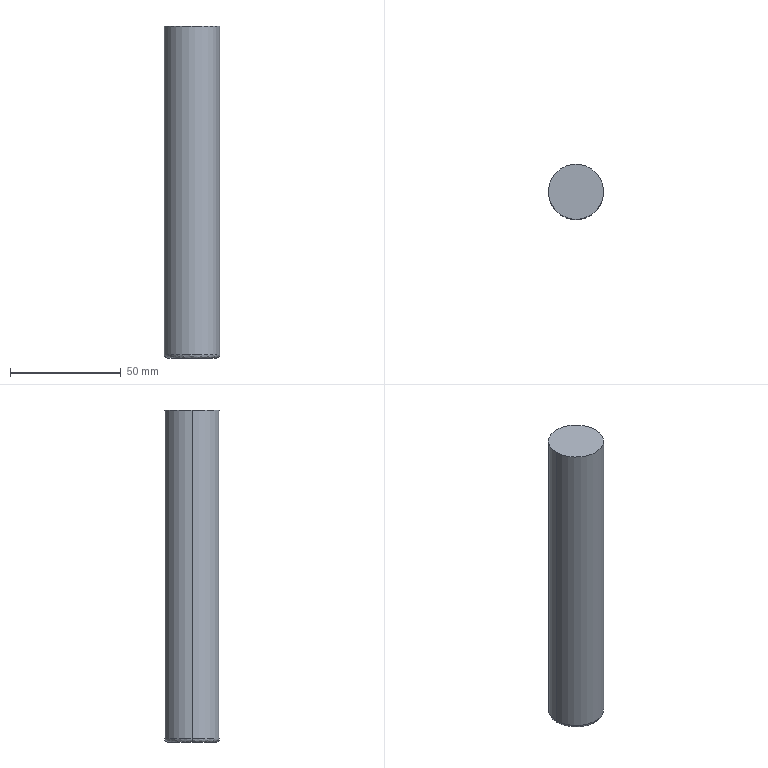Part | SolidWorks | features BaseBody 1 | 1 solid | 27 faces | box 25 x 25 x 150 mm | volume 71513 mm3 | cylinder 17 | spline 5 | plane 5 | commonest cylinder face diameters 10 x15 25 x2